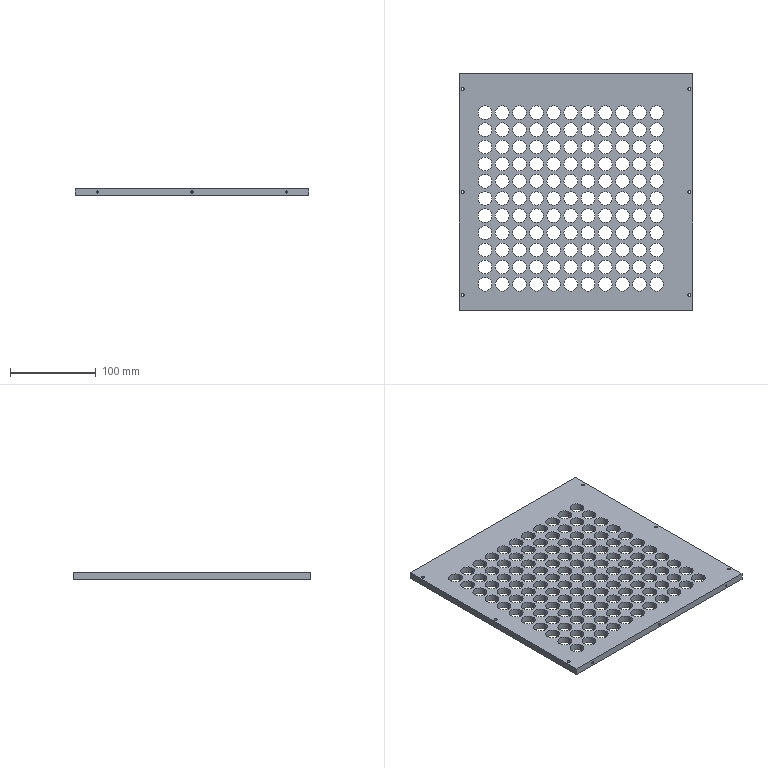Part | STEP file | CA-10-007Lift Stop Plate3_Default | 1 solid | 302 faces | box 272 x 275 x 8 mm | volume 402632 mm3 | cylinder 278 | cone 12 | plane 12 | commonest cylinder face diameters 16 x242 2.5 x12 3.4 x12 5.5 x12